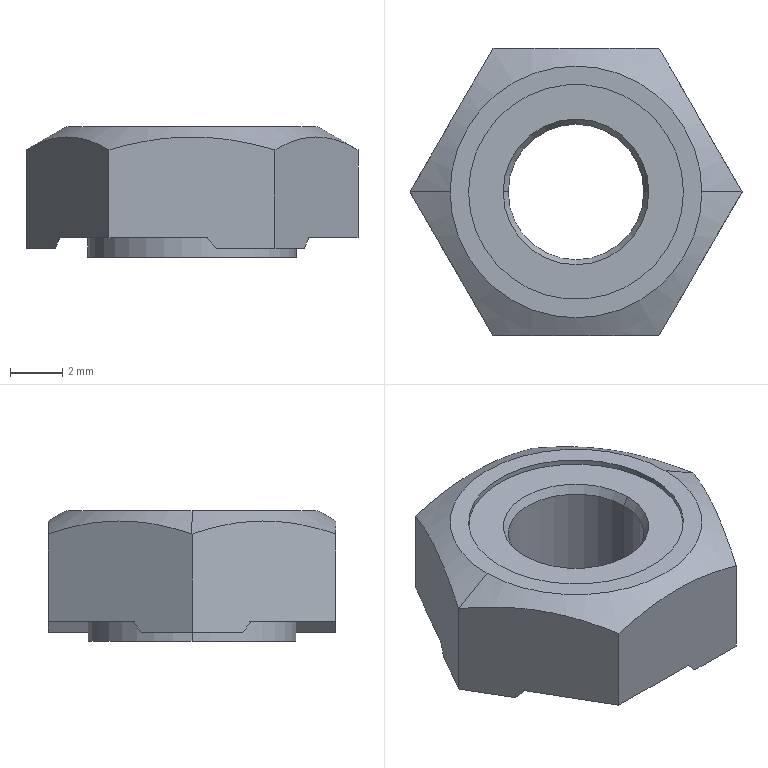Part | STEP file | hexagon weld nuts gb_GB_FASTENER_NUT_JSCN M6-N | 1 solid | 28 faces | box 12.702 x 11 x 5 mm | volume 362.782 mm3 | plane 16 | cone 6 | cylinder 6 | commonest cylinder face diameters 5.188 x2 7.96 x2 8.22 x2